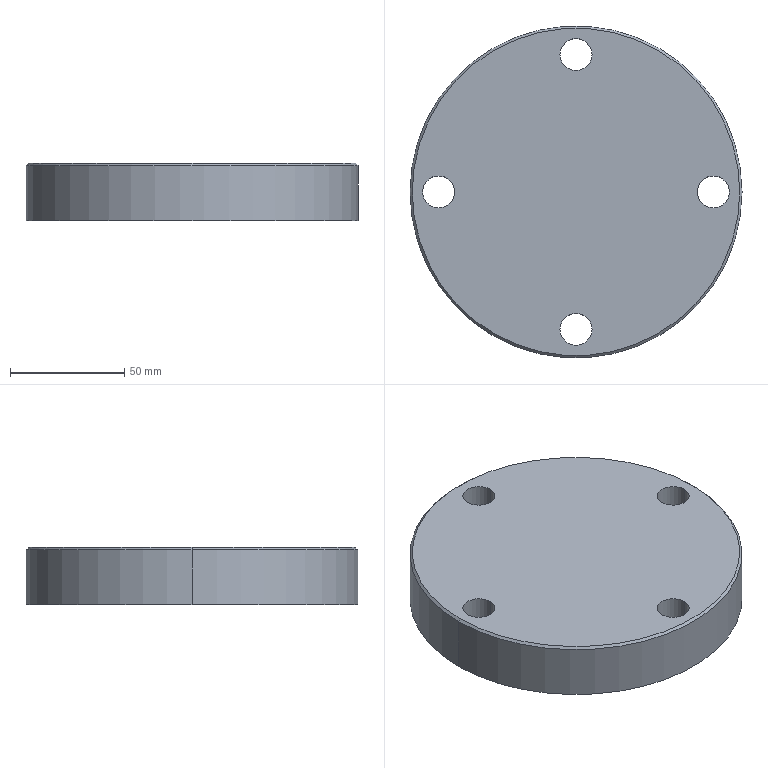Part | SolidWorks | features Chamfer 2, ICE 2, Extrusion 1 | 1 solid | 25 faces | box 145 x 145 x 25 mm | volume 302931 mm3 | cylinder 13 | plane 7 | cone 5 | commonest cylinder face diameters 14 x8 97 x3 145 x2
STEP:
#1=CARTESIAN_POINT('',(-48.5,0.,1.));
#2=VERTEX_POINT('',#1);
#3=CARTESIAN_POINT('',(-32.5,36.,1.));
#4=VERTEX_POINT('',#3);
#5=CARTESIAN_POINT('',(0.,0.,1.));
#6=DIRECTION('',(0.,0.,-1.));
#7=DIRECTION('',(1.,0.,0.));
#8=AXIS2_PLACEMENT_3D('',#5,#6,#7);
#9=CIRCLE('',#8,48.5);
#10=EDGE_CURVE('',#2,#4,#9,.T.);
#11=ORIENTED_EDGE('',*,*,#10,.F.);
#12=CARTESIAN_POINT('',(-49.5,0.,0.));
#13=VERTEX_POINT('',#12);
#14=CARTESIAN_POINT('',(-48.5,0.,1.));
#15=DIRECTION('',(-0.7071,0.,-0.7071));
#16=VECTOR('',#15,1000.);
#17=LINE('',#14,#16);
#18=EDGE_CURVE('',#2,#13,#17,.T.);
#19=ORIENTED_EDGE('',*,*,#18,.T.);
#20=CARTESIAN_POINT('',(-32.882,37.,0.));
#21=VERTEX_POINT('',#20);
#22=CARTESIAN_POINT('',(0.,0.,0.));
#23=DIRECTION('',(0.,0.,1.));
#24=DIRECTION('',(1.,0.,0.));
#25=AXIS2_PLACEMENT_3D('',#22,#23,#24);
#26=CIRCLE('',#25,49.5);
#27=EDGE_CURVE('',#21,#13,#26,.T.);
#28=ORIENTED_EDGE('',*,*,#27,.F.);
#29=CARTESIAN_POINT('',(-32.5,36.,1.));
#30=CARTESIAN_POINT('',(-32.628,36.333,0.6668));
#31=CARTESIAN_POINT('',(-32.756,36.667,0.3335));
#32=CARTESIAN_POINT('',(-32.882,37.,0.));
#33=B_SPLINE_CURVE_WITH_KNOTS('',3,(#29,#30,#31,#32),.UNSPECIFIED.,.F.,.F.,(4,4),(0.,0.001465),.UNSPECIFIED.);
#34=EDGE_CURVE('',#4,#21,#33,.T.);
#35=ORIENTED_EDGE('',*,*,#34,.F.);
#36=EDGE_LOOP('',(#11,#19,#28,#35));
#37=FACE_OUTER_BOUND('',#36,.T.);
#38=CARTESIAN_POINT('',(0.,0.,1.));
#39=DIRECTION('',(0.,0.,-1.));
#40=DIRECTION('',(-1.,0.,0.));
#41=AXIS2_PLACEMENT_3D('',#38,#39,#40);
#42=CONICAL_SURFACE('',#41,48.5,0.7854);
#43=ADVANCED_FACE('',(#37),#42,.F.);
#44=CARTESIAN_POINT('',(71.5,0.,25.));
#45=VERTEX_POINT('',#44);
#46=CARTESIAN_POINT('',(-71.5,0.,25.));
#47=VERTEX_POINT('',#46);
#48=CARTESIAN_POINT('',(0.,0.,25.));
#49=DIRECTION('',(0.,0.,1.));
#50=DIRECTION('',(1.,0.,0.));
#51=AXIS2_PLACEMENT_3D('',#48,#49,#50);
#52=CIRCLE('',#51,71.5);
#53=EDGE_CURVE('',#45,#47,#52,.T.);
#54=ORIENTED_EDGE('',*,*,#53,.F.);
#55=CARTESIAN_POINT('',(72.5,0.,24.));
#56=VERTEX_POINT('',#55);
#57=CARTESIAN_POINT('',(71.5,0.,25.));
#58=DIRECTION('',(0.7071,0.,-0.7071));
#59=VECTOR('',#58,1000.);
#60=LINE('',#57,#59);
#61=EDGE_CURVE('',#45,#56,#60,.T.);
#62=ORIENTED_EDGE('',*,*,#61,.T.);
#63=CARTESIAN_POINT('',(-72.5,0.,24.));
#64=VERTEX_POINT('',#63);
#65=CARTESIAN_POINT('',(0.,0.,24.));
#66=DIRECTION('',(0.,0.,-1.));
#67=DIRECTION('',(1.,0.,0.));
#68=AXIS2_PLACEMENT_3D('',#65,#66,#67);
#69=CIRCLE('',#68,72.5);
#70=EDGE_CURVE('',#64,#56,#69,.T.);
#71=ORIENTED_EDGE('',*,*,#70,.F.);
#72=CARTESIAN_POINT('',(-71.5,0.,25.));
#73=DIRECTION('',(-0.7071,0.,-0.7071));
#74=VECTOR('',#73,1000.);
#75=LINE('',#72,#74);
#76=EDGE_CURVE('',#47,#64,#75,.T.);
#77=ORIENTED_EDGE('',*,*,#76,.F.);
#78=EDGE_LOOP('',(#54,#62,#71,#77));
#79=FACE_OUTER_BOUND('',#78,.T.);
#80=CARTESIAN_POINT('',(0.,0.,25.));
#81=DIRECTION('',(0.,0.,-1.));
#82=DIRECTION('',(-1.,0.,0.));
#83=AXIS2_PLACEMENT_3D('',#80,#81,#82);
#84=CONICAL_SURFACE('',#83,71.5,0.7854);
#85=ADVANCED_FACE('',(#79),#84,.T.);
#86=CARTESIAN_POINT('',(-48.5,0.,15.));
#87=VERTEX_POINT('',#86);
#88=CARTESIAN_POINT('',(-32.5,36.,15.));
#89=VERTEX_POINT('',#88);
#90=CARTESIAN_POINT('',(0.,0.,15.));
#91=DIRECTION('',(0.,0.,-1.));
#92=DIRECTION('',(-1.,0.,0.));
#93=AXIS2_PLACEMENT_3D('',#90,#91,#92);
#94=CIRCLE('',#93,48.5);
#95=EDGE_CURVE('',#87,#89,#94,.T.);
#96=ORIENTED_EDGE('',*,*,#95,.F.);
#97=CARTESIAN_POINT('',(-48.5,0.,15.));
#98=DIRECTION('',(0.,0.,-1.));
#99=VECTOR('',#98,1000.);
#100=LINE('',#97,#99);
#101=EDGE_CURVE('',#87,#2,#100,.T.);
#102=ORIENTED_EDGE('',*,*,#101,.T.);
#103=ORIENTED_EDGE('',*,*,#10,.T.);
#104=CARTESIAN_POINT('',(-32.5,36.,15.));
#105=DIRECTION('',(0.,0.,-1.));
#106=VECTOR('',#105,1000.);
#107=LINE('',#104,#106);
#108=EDGE_CURVE('',#89,#4,#107,.T.);
#109=ORIENTED_EDGE('',*,*,#108,.F.);
#110=EDGE_LOOP('',(#96,#102,#103,#109));
#111=FACE_OUTER_BOUND('',#110,.T.);
#112=CARTESIAN_POINT('',(0.,0.,15.));
#113=DIRECTION('',(0.,0.,-1.));
#114=DIRECTION('',(-1.,0.,0.));
#115=AXIS2_PLACEMENT_3D('',#112,#113,#114);
#116=CYLINDRICAL_SURFACE('',#115,48.5);
#117=ADVANCED_FACE('',(#111),#116,.F.);
#118=CARTESIAN_POINT('',(53.,0.,0.));
#119=VERTEX_POINT('',#118);
#120=CARTESIAN_POINT('',(67.,0.,0.));
#121=VERTEX_POINT('',#120);
#122=CARTESIAN_POINT('',(60.,0.,0.));
#123=DIRECTION('',(0.,0.,1.));
#124=DIRECTION('',(1.,0.,0.));
#125=AXIS2_PLACEMENT_3D('',#122,#123,#124);
#126=CIRCLE('',#125,7.);
#127=EDGE_CURVE('',#119,#121,#126,.T.);
#128=ORIENTED_EDGE('',*,*,#127,.F.);
#129=CARTESIAN_POINT('',(53.,0.,25.));
#130=VERTEX_POINT('',#129);
#131=CARTESIAN_POINT('',(53.,0.,0.));
#132=DIRECTION('',(0.,0.,1.));
#133=VECTOR('',#132,1000.);
#134=LINE('',#131,#133);
#135=EDGE_CURVE('',#119,#130,#134,.T.);
#136=ORIENTED_EDGE('',*,*,#135,.T.);
#137=CARTESIAN_POINT('',(67.,0.,25.));
#138=VERTEX_POINT('',#137);
#139=CARTESIAN_POINT('',(60.,0.,25.));
#140=DIRECTION('',(0.,0.,1.));
#141=DIRECTION('',(1.,0.,0.));
#142=AXIS2_PLACEMENT_3D('',#139,#140,#141);
#143=CIRCLE('',#142,7.);
#144=EDGE_CURVE('',#130,#138,#143,.T.);
#145=ORIENTED_EDGE('',*,*,#144,.T.);
#146=CARTESIAN_POINT('',(67.,0.,0.));
#147=DIRECTION('',(0.,0.,1.));
#148=VECTOR('',#147,1000.);
#149=LINE('',#146,#148);
#150=EDGE_CURVE('',#121,#138,#149,.T.);
#151=ORIENTED_EDGE('',*,*,#150,.F.);
#152=EDGE_LOOP('',(#128,#136,#145,#151));
#153=FACE_OUTER_BOUND('',#152,.T.);
#154=CARTESIAN_POINT('',(60.,0.,0.));
#155=DIRECTION('',(0.,0.,1.));
#156=DIRECTION('',(1.,0.,0.));
#157=AXIS2_PLACEMENT_3D('',#154,#155,#156);
#158=CYLINDRICAL_SURFACE('',#157,7.);
#159=ADVANCED_FACE('',(#153),#158,.F.);
#160=CARTESIAN_POINT('',(-7.,-60.,0.));
#161=VERTEX_POINT('',#160);
#162=CARTESIAN_POINT('',(7.,-60.,0.));
#163=VERTEX_POINT('',#162);
#164=CARTESIAN_POINT('',(0.,-60.,0.));
#165=DIRECTION('',(0.,0.,1.));
#166=DIRECTION('',(1.,0.,0.));
#167=AXIS2_PLACEMENT_3D('',#164,#165,#166);
#168=CIRCLE('',#167,7.);
#169=EDGE_CURVE('',#161,#163,#168,.T.);
#170=ORIENTED_EDGE('',*,*,#169,.F.);
#171=CARTESIAN_POINT('',(-7.,-60.,25.));
#172=VERTEX_POINT('',#171);
#173=CARTESIAN_POINT('',(-7.,-60.,0.));
#174=DIRECTION('',(0.,0.,1.));
#175=VECTOR('',#174,1000.);
#176=LINE('',#173,#175);
#177=EDGE_CURVE('',#161,#172,#176,.T.);
#178=ORIENTED_EDGE('',*,*,#177,.T.);
#179=CARTESIAN_POINT('',(7.,-60.,25.));
#180=VERTEX_POINT('',#179);
#181=CARTESIAN_POINT('',(0.,-60.,25.));
#182=DIRECTION('',(0.,0.,1.));
#183=DIRECTION('',(1.,0.,0.));
#184=AXIS2_PLACEMENT_3D('',#181,#182,#183);
#185=CIRCLE('',#184,7.);
#186=EDGE_CURVE('',#172,#180,#185,.T.);
#187=ORIENTED_EDGE('',*,*,#186,.T.);
#188=CARTESIAN_POINT('',(7.,-60.,0.));
#189=DIRECTION('',(0.,0.,1.));
#190=VECTOR('',#189,1000.);
#191=LINE('',#188,#190);
#192=EDGE_CURVE('',#163,#180,#191,.T.);
#193=ORIENTED_EDGE('',*,*,#192,.F.);
#194=EDGE_LOOP('',(#170,#178,#187,#193));
#195=FACE_OUTER_BOUND('',#194,.T.);
#196=CARTESIAN_POINT('',(0.,-60.,0.));
#197=DIRECTION('',(0.,0.,1.));
#198=DIRECTION('',(1.,0.,0.));
#199=AXIS2_PLACEMENT_3D('',#196,#197,#198);
#200=CYLINDRICAL_SURFACE('',#199,7.);
#201=ADVANCED_FACE('',(#195),#200,.F.);
#202=CARTESIAN_POINT('',(-67.,0.,0.));
#203=VERTEX_POINT('',#202);
#204=CARTESIAN_POINT('',(-53.,0.,0.));
#205=VERTEX_POINT('',#204);
#206=CARTESIAN_POINT('',(-60.,0.,0.));
#207=DIRECTION('',(0.,0.,1.));
#208=DIRECTION('',(1.,0.,0.));
#209=AXIS2_PLACEMENT_3D('',#206,#207,#208);
#210=CIRCLE('',#209,7.);
#211=EDGE_CURVE('',#203,#205,#210,.T.);
#212=ORIENTED_EDGE('',*,*,#211,.F.);
#213=CARTESIAN_POINT('',(-67.,0.,25.));
#214=VERTEX_POINT('',#213);
#215=CARTESIAN_POINT('',(-67.,0.,0.));
#216=DIRECTION('',(0.,0.,1.));
#217=VECTOR('',#216,1000.);
#218=LINE('',#215,#217);
#219=EDGE_CURVE('',#203,#214,#218,.T.);
#220=ORIENTED_EDGE('',*,*,#219,.T.);
#221=CARTESIAN_POINT('',(-53.,0.,25.));
#222=VERTEX_POINT('',#221);
#223=CARTESIAN_POINT('',(-60.,0.,25.));
#224=DIRECTION('',(0.,0.,1.));
#225=DIRECTION('',(1.,0.,0.));
#226=AXIS2_PLACEMENT_3D('',#223,#224,#225);
#227=CIRCLE('',#226,7.);
#228=EDGE_CURVE('',#214,#222,#227,.T.);
#229=ORIENTED_EDGE('',*,*,#228,.T.);
#230=CARTESIAN_POINT('',(-53.,0.,0.));
#231=DIRECTION('',(0.,0.,1.));
#232=VECTOR('',#231,1000.);
#233=LINE('',#230,#232);
#234=EDGE_CURVE('',#205,#222,#233,.T.);
#235=ORIENTED_EDGE('',*,*,#234,.F.);
#236=EDGE_LOOP('',(#212,#220,#229,#235));
#237=FACE_OUTER_BOUND('',#236,.T.);
#238=CARTESIAN_POINT('',(-60.,0.,0.));
#239=DIRECTION('',(0.,0.,1.));
#240=DIRECTION('',(1.,0.,0.));
#241=AXIS2_PLACEMENT_3D('',#238,#239,#240);
#242=CYLINDRICAL_SURFACE('',#241,7.);
#243=ADVANCED_FACE('',(#237),#242,.F.);
#244=CARTESIAN_POINT('',(-7.,60.,0.));
#245=VERTEX_POINT('',#244);
#246=CARTESIAN_POINT('',(7.,60.,0.));
#247=VERTEX_POINT('',#246);
#248=CARTESIAN_POINT('',(0.,60.,0.));
#249=DIRECTION('',(0.,0.,1.));
#250=DIRECTION('',(1.,0.,0.));
#251=AXIS2_PLACEMENT_3D('',#248,#249,#250);
#252=CIRCLE('',#251,7.);
#253=EDGE_CURVE('',#245,#247,#252,.T.);
#254=ORIENTED_EDGE('',*,*,#253,.F.);
#255=CARTESIAN_POINT('',(-7.,60.,25.));
#256=VERTEX_POINT('',#255);
#257=CARTESIAN_POINT('',(-7.,60.,0.));
#258=DIRECTION('',(0.,0.,1.));
#259=VECTOR('',#258,1000.);
#260=LINE('',#257,#259);
#261=EDGE_CURVE('',#245,#256,#260,.T.);
#262=ORIENTED_EDGE('',*,*,#261,.T.);
#263=CARTESIAN_POINT('',(7.,60.,25.));
#264=VERTEX_POINT('',#263);
#265=CARTESIAN_POINT('',(0.,60.,25.));
#266=DIRECTION('',(0.,0.,1.));
#267=DIRECTION('',(1.,0.,0.));
#268=AXIS2_PLACEMENT_3D('',#265,#266,#267);
#269=CIRCLE('',#268,7.);
#270=EDGE_CURVE('',#256,#264,#269,.T.);
#271=ORIENTED_EDGE('',*,*,#270,.T.);
#272=CARTESIAN_POINT('',(7.,60.,0.));
#273=DIRECTION('',(0.,0.,1.));
#274=VECTOR('',#273,1000.);
#275=LINE('',#272,#274);
#276=EDGE_CURVE('',#247,#264,#275,.T.);
#277=ORIENTED_EDGE('',*,*,#276,.F.);
#278=EDGE_LOOP('',(#254,#262,#271,#277));
#279=FACE_OUTER_BOUND('',#278,.T.);
#280=CARTESIAN_POINT('',(0.,60.,0.));
#281=DIRECTION('',(0.,0.,1.));
#282=DIRECTION('',(1.,0.,0.));
#283=AXIS2_PLACEMENT_3D('',#280,#281,#282);
#284=CYLINDRICAL_SURFACE('',#283,7.);
#285=ADVANCED_FACE('',(#279),#284,.F.);
#286=ORIENTED_EDGE('',*,*,#70,.T.);
#287=CARTESIAN_POINT('',(72.5,0.,0.));
#288=VERTEX_POINT('',#287);
#289=CARTESIAN_POINT('',(72.5,0.,25.));
#290=DIRECTION('',(0.,0.,-1.));
#291=VECTOR('',#290,1000.);
#292=LINE('',#289,#291);
#293=EDGE_CURVE('',#56,#288,#292,.T.);
#294=ORIENTED_EDGE('',*,*,#293,.T.);
#295=CARTESIAN_POINT('',(-72.5,0.,0.));
#296=VERTEX_POINT('',#295);
#297=CARTESIAN_POINT('',(0.,0.,0.));
#298=DIRECTION('',(0.,0.,1.));
#299=DIRECTION('',(1.,0.,0.));
#300=AXIS2_PLACEMENT_3D('',#297,#298,#299);
#301=CIRCLE('',#300,72.5);
#302=EDGE_CURVE('',#288,#296,#301,.T.);
#303=ORIENTED_EDGE('',*,*,#302,.T.);
#304=CARTESIAN_POINT('',(-72.5,0.,25.));
#305=DIRECTION('',(0.,0.,-1.));
#306=VECTOR('',#305,1000.);
#307=LINE('',#304,#306);
#308=EDGE_CURVE('',#64,#296,#307,.T.);
#309=ORIENTED_EDGE('',*,*,#308,.F.);
#310=EDGE_LOOP('',(#286,#294,#303,#309));
#311=FACE_OUTER_BOUND('',#310,.T.);
#312=CARTESIAN_POINT('',(0.,0.,25.));
#313=DIRECTION('',(0.,0.,-1.));
#314=DIRECTION('',(-1.,0.,0.));
#315=AXIS2_PLACEMENT_3D('',#312,#313,#314);
#316=CYLINDRICAL_SURFACE('',#315,72.5);
#317=ADVANCED_FACE('',(#311),#316,.T.);
#318=ORIENTED_EDGE('',*,*,#293,.F.);
#319=CARTESIAN_POINT('',(0.,0.,24.));
#320=DIRECTION('',(0.,0.,-1.));
#321=DIRECTION('',(1.,0.,0.));
#322=AXIS2_PLACEMENT_3D('',#319,#320,#321);
#323=CIRCLE('',#322,72.5);
#324=EDGE_CURVE('',#56,#64,#323,.T.);
#325=ORIENTED_EDGE('',*,*,#324,.T.);
#326=ORIENTED_EDGE('',*,*,#308,.T.);
#327=CARTESIAN_POINT('',(0.,0.,0.));
#328=DIRECTION('',(0.,0.,1.));
#329=DIRECTION('',(1.,0.,0.));
#330=AXIS2_PLACEMENT_3D('',#327,#328,#329);
#331=CIRCLE('',#330,72.5);
#332=EDGE_CURVE('',#296,#288,#331,.T.);
#333=ORIENTED_EDGE('',*,*,#332,.T.);
#334=EDGE_LOOP('',(#318,#325,#326,#333));
#335=FACE_OUTER_BOUND('',#334,.T.);
#336=CARTESIAN_POINT('',(0.,0.,25.));
#337=DIRECTION('',(0.,0.,-1.));
#338=DIRECTION('',(-1.,0.,0.));
#339=AXIS2_PLACEMENT_3D('',#336,#337,#338);
#340=CYLINDRICAL_SURFACE('',#339,72.5);
#341=ADVANCED_FACE('',(#335),#340,.T.);
#342=CARTESIAN_POINT('',(0.,0.,25.));
#343=DIRECTION('',(0.,0.,1.));
#344=DIRECTION('',(1.,0.,0.));
#345=AXIS2_PLACEMENT_3D('',#342,#343,#344);
#346=CIRCLE('',#345,71.5);
#347=EDGE_CURVE('',#47,#45,#346,.T.);
#348=ORIENTED_EDGE('',*,*,#347,.T.);
#349=ORIENTED_EDGE('',*,*,#53,.T.);
#350=EDGE_LOOP('',(#348,#349));
#351=FACE_OUTER_BOUND('',#350,.T.);
#352=CARTESIAN_POINT('',(60.,0.,25.));
#353=DIRECTION('',(0.,0.,1.));
#354=DIRECTION('',(1.,0.,0.));
#355=AXIS2_PLACEMENT_3D('',#352,#353,#354);
#356=CIRCLE('',#355,7.);
#357=EDGE_CURVE('',#138,#130,#356,.T.);
#358=ORIENTED_EDGE('',*,*,#357,.F.);
#359=ORIENTED_EDGE('',*,*,#144,.F.);
#360=EDGE_LOOP('',(#358,#359));
#361=FACE_BOUND('',#360,.T.);
#362=CARTESIAN_POINT('',(0.,-60.,25.));
#363=DIRECTION('',(0.,0.,1.));
#364=DIRECTION('',(1.,0.,0.));
#365=AXIS2_PLACEMENT_3D('',#362,#363,#364);
#366=CIRCLE('',#365,7.);
#367=EDGE_CURVE('',#180,#172,#366,.T.);
#368=ORIENTED_EDGE('',*,*,#367,.F.);
#369=ORIENTED_EDGE('',*,*,#186,.F.);
#370=EDGE_LOOP('',(#368,#369));
#371=FACE_BOUND('',#370,.T.);
#372=CARTESIAN_POINT('',(-60.,0.,25.));
#373=DIRECTION('',(0.,0.,1.));
#374=DIRECTION('',(1.,0.,0.));
#375=AXIS2_PLACEMENT_3D('',#372,#373,#374);
#376=CIRCLE('',#375,7.);
#377=EDGE_CURVE('',#222,#214,#376,.T.);
#378=ORIENTED_EDGE('',*,*,#377,.F.);
#379=ORIENTED_EDGE('',*,*,#228,.F.);
#380=EDGE_LOOP('',(#378,#379));
#381=FACE_BOUND('',#380,.T.);
#382=CARTESIAN_POINT('',(0.,60.,25.));
#383=DIRECTION('',(0.,0.,1.));
#384=DIRECTION('',(1.,0.,0.));
#385=AXIS2_PLACEMENT_3D('',#382,#383,#384);
#386=CIRCLE('',#385,7.);
#387=EDGE_CURVE('',#264,#256,#386,.T.);
#388=ORIENTED_EDGE('',*,*,#387,.F.);
#389=ORIENTED_EDGE('',*,*,#270,.F.);
#390=EDGE_LOOP('',(#388,#389));
#391=FACE_BOUND('',#390,.T.);
#392=CARTESIAN_POINT('',(0.,0.,25.));
#393=DIRECTION('',(0.,0.,1.));
#394=DIRECTION('',(1.,0.,0.));
#395=AXIS2_PLACEMENT_3D('',#392,#393,#394);
#396=PLANE('',#395);
#397=ADVANCED_FACE('',(#351,#361,#371,#381,#391),#396,.T.);
#398=CARTESIAN_POINT('',(32.882,-37.,0.));
#399=VERTEX_POINT('',#398);
#400=CARTESIAN_POINT('',(32.882,37.,0.));
#401=VERTEX_POINT('',#400);
#402=CARTESIAN_POINT('',(0.,0.,0.));
#403=DIRECTION('',(0.,0.,1.));
#404=DIRECTION('',(1.,0.,0.));
#405=AXIS2_PLACEMENT_3D('',#402,#403,#404);
#406=CIRCLE('',#405,49.5);
#407=EDGE_CURVE('',#399,#401,#406,.T.);
#408=ORIENTED_EDGE('',*,*,#407,.T.);
#409=CARTESIAN_POINT('',(0.,37.,0.));
#410=DIRECTION('',(-1.,0.,0.));
#411=VECTOR('',#410,1000.);
#412=LINE('',#409,#411);
#413=EDGE_CURVE('',#401,#21,#412,.T.);
#414=ORIENTED_EDGE('',*,*,#413,.T.);
#415=ORIENTED_EDGE('',*,*,#27,.T.);
#416=CARTESIAN_POINT('',(-32.882,-37.,0.));
#417=VERTEX_POINT('',#416);
#418=CARTESIAN_POINT('',(0.,0.,0.));
#419=DIRECTION('',(0.,0.,1.));
#420=DIRECTION('',(1.,0.,0.));
#421=AXIS2_PLACEMENT_3D('',#418,#419,#420);
#422=CIRCLE('',#421,49.5);
#423=EDGE_CURVE('',#13,#417,#422,.T.);
#424=ORIENTED_EDGE('',*,*,#423,.T.);
#425=CARTESIAN_POINT('',(0.,-37.,0.));
#426=DIRECTION('',(1.,0.,0.));
#427=VECTOR('',#426,1000.);
#428=LINE('',#425,#427);
#429=EDGE_CURVE('',#417,#399,#428,.T.);
#430=ORIENTED_EDGE('',*,*,#429,.T.);
#431=EDGE_LOOP('',(#408,#414,#415,#424,#430));
#432=FACE_BOUND('',#431,.T.);
#433=CARTESIAN_POINT('',(60.,0.,0.));
#434=DIRECTION('',(0.,0.,1.));
#435=DIRECTION('',(1.,0.,0.));
#436=AXIS2_PLACEMENT_3D('',#433,#434,#435);
#437=CIRCLE('',#436,7.);
#438=EDGE_CURVE('',#121,#119,#437,.T.);
#439=ORIENTED_EDGE('',*,*,#438,.T.);
#440=ORIENTED_EDGE('',*,*,#127,.T.);
#441=EDGE_LOOP('',(#439,#440));
#442=FACE_BOUND('',#441,.T.);
#443=CARTESIAN_POINT('',(0.,-60.,0.));
#444=DIRECTION('',(0.,0.,1.));
#445=DIRECTION('',(1.,0.,0.));
#446=AXIS2_PLACEMENT_3D('',#443,#444,#445);
#447=CIRCLE('',#446,7.);
#448=EDGE_CURVE('',#163,#161,#447,.T.);
#449=ORIENTED_EDGE('',*,*,#448,.T.);
#450=ORIENTED_EDGE('',*,*,#169,.T.);
#451=EDGE_LOOP('',(#449,#450));
#452=FACE_BOUND('',#451,.T.);
#453=CARTESIAN_POINT('',(-60.,0.,0.));
#454=DIRECTION('',(0.,0.,1.));
#455=DIRECTION('',(1.,0.,0.));
#456=AXIS2_PLACEMENT_3D('',#453,#454,#455);
#457=CIRCLE('',#456,7.);
#458=EDGE_CURVE('',#205,#203,#457,.T.);
#459=ORIENTED_EDGE('',*,*,#458,.T.);
#460=ORIENTED_EDGE('',*,*,#211,.T.);
#461=EDGE_LOOP('',(#459,#460));
#462=FACE_BOUND('',#461,.T.);
#463=CARTESIAN_POINT('',(0.,60.,0.));
#464=DIRECTION('',(0.,0.,1.));
#465=DIRECTION('',(1.,0.,0.));
#466=AXIS2_PLACEMENT_3D('',#463,#464,#465);
#467=CIRCLE('',#466,7.);
#468=EDGE_CURVE('',#247,#245,#467,.T.);
#469=ORIENTED_EDGE('',*,*,#468,.T.);
#470=ORIENTED_EDGE('',*,*,#253,.T.);
#471=EDGE_LOOP('',(#469,#470));
#472=FACE_BOUND('',#471,.T.);
#473=ORIENTED_EDGE('',*,*,#332,.F.);
#474=ORIENTED_EDGE('',*,*,#302,.F.);
#475=EDGE_LOOP('',(#473,#474));
#476=FACE_OUTER_BOUND('',#475,.T.);
#477=CARTESIAN_POINT('',(0.,0.,0.));
#478=DIRECTION('',(0.,0.,1.));
#479=DIRECTION('',(1.,0.,0.));
#480=AXIS2_PLACEMENT_3D('',#477,#478,#479);
#481=PLANE('',#480);
#482=ADVANCED_FACE('',(#432,#442,#452,#462,#472,#476),#481,.F.);
#483=ORIENTED_EDGE('',*,*,#261,.F.);
#484=ORIENTED_EDGE('',*,*,#468,.F.);
#485=ORIENTED_EDGE('',*,*,#276,.T.);
#486=ORIENTED_EDGE('',*,*,#387,.T.);
#487=EDGE_LOOP('',(#483,#484,#485,#486));
#488=FACE_OUTER_BOUND('',#487,.T.);
#489=CARTESIAN_POINT('',(0.,60.,0.));
#490=DIRECTION('',(0.,0.,1.));
#491=DIRECTION('',(1.,0.,0.));
#492=AXIS2_PLACEMENT_3D('',#489,#490,#491);
#493=CYLINDRICAL_SURFACE('',#492,7.);
#494=ADVANCED_FACE('',(#488),#493,.F.);
#495=ORIENTED_EDGE('',*,*,#219,.F.);
#496=ORIENTED_EDGE('',*,*,#458,.F.);
#497=ORIENTED_EDGE('',*,*,#234,.T.);
#498=ORIENTED_EDGE('',*,*,#377,.T.);
#499=EDGE_LOOP('',(#495,#496,#497,#498));
#500=FACE_OUTER_BOUND('',#499,.T.);
#501=CARTESIAN_POINT('',(-60.,0.,0.));
#502=DIRECTION('',(0.,0.,1.));
#503=DIRECTION('',(1.,0.,0.));
#504=AXIS2_PLACEMENT_3D('',#501,#502,#503);
#505=CYLINDRICAL_SURFACE('',#504,7.);
#506=ADVANCED_FACE('',(#500),#505,.F.);
#507=ORIENTED_EDGE('',*,*,#177,.F.);
#508=ORIENTED_EDGE('',*,*,#448,.F.);
#509=ORIENTED_EDGE('',*,*,#192,.T.);
#510=ORIENTED_EDGE('',*,*,#367,.T.);
#511=EDGE_LOOP('',(#507,#508,#509,#510));
#512=FACE_OUTER_BOUND('',#511,.T.);
#513=CARTESIAN_POINT('',(0.,-60.,0.));
#514=DIRECTION('',(0.,0.,1.));
#515=DIRECTION('',(1.,0.,0.));
#516=AXIS2_PLACEMENT_3D('',#513,#514,#515);
#517=CYLINDRICAL_SURFACE('',#516,7.);
#518=ADVANCED_FACE('',(#512),#517,.F.);
#519=ORIENTED_EDGE('',*,*,#135,.F.);
#520=ORIENTED_EDGE('',*,*,#438,.F.);
#521=ORIENTED_EDGE('',*,*,#150,.T.);
#522=ORIENTED_EDGE('',*,*,#357,.T.);
#523=EDGE_LOOP('',(#519,#520,#521,#522));
#524=FACE_OUTER_BOUND('',#523,.T.);
#525=CARTESIAN_POINT('',(60.,0.,0.));
#526=DIRECTION('',(0.,0.,1.));
#527=DIRECTION('',(1.,0.,0.));
#528=AXIS2_PLACEMENT_3D('',#525,#526,#527);
#529=CYLINDRICAL_SURFACE('',#528,7.);
#530=ADVANCED_FACE('',(#524),#529,.F.);
#531=CARTESIAN_POINT('',(32.5,36.,15.));
#532=VERTEX_POINT('',#531);
#533=CARTESIAN_POINT('',(32.5,36.,1.));
#534=VERTEX_POINT('',#533);
#535=CARTESIAN_POINT('',(32.5,36.,15.));
#536=DIRECTION('',(0.,0.,-1.));
#537=VECTOR('',#536,1000.);
#538=LINE('',#535,#537);
#539=EDGE_CURVE('',#532,#534,#538,.T.);
#540=ORIENTED_EDGE('',*,*,#539,.T.);
#541=CARTESIAN_POINT('',(32.5,-36.,1.));
#542=VERTEX_POINT('',#541);
#543=CARTESIAN_POINT('',(0.,0.,1.));
#544=DIRECTION('',(0.,0.,-1.));
#545=DIRECTION('',(1.,0.,0.));
#546=AXIS2_PLACEMENT_3D('',#543,#544,#545);
#547=CIRCLE('',#546,48.5);
#548=EDGE_CURVE('',#534,#542,#547,.T.);
#549=ORIENTED_EDGE('',*,*,#548,.T.);
#550=CARTESIAN_POINT('',(32.5,-36.,15.));
#551=VERTEX_POINT('',#550);
#552=CARTESIAN_POINT('',(32.5,-36.,15.));
#553=DIRECTION('',(0.,0.,-1.));
#554=VECTOR('',#553,1000.);
#555=LINE('',#552,#554);
#556=EDGE_CURVE('',#551,#542,#555,.T.);
#557=ORIENTED_EDGE('',*,*,#556,.F.);
#558=CARTESIAN_POINT('',(0.,0.,15.));
#559=DIRECTION('',(0.,0.,-1.));
#560=DIRECTION('',(-1.,0.,0.));
#561=AXIS2_PLACEMENT_3D('',#558,#559,#560);
#562=CIRCLE('',#561,48.5);
#563=EDGE_CURVE('',#532,#551,#562,.T.);
#564=ORIENTED_EDGE('',*,*,#563,.F.);
#565=EDGE_LOOP('',(#540,#549,#557,#564));
#566=FACE_OUTER_BOUND('',#565,.T.);
#567=CARTESIAN_POINT('',(0.,0.,15.));
#568=DIRECTION('',(0.,0.,-1.));
#569=DIRECTION('',(-1.,0.,0.));
#570=AXIS2_PLACEMENT_3D('',#567,#568,#569);
#571=CYLINDRICAL_SURFACE('',#570,48.5);
#572=ADVANCED_FACE('',(#566),#571,.F.);
#573=ORIENTED_EDGE('',*,*,#108,.T.);
#574=CARTESIAN_POINT('',(32.5,36.,1.));
#575=DIRECTION('',(1.,0.,0.));
#576=VECTOR('',#575,1000.);
#577=LINE('',#574,#576);
#578=EDGE_CURVE('',#4,#534,#577,.T.);
#579=ORIENTED_EDGE('',*,*,#578,.T.);
#580=ORIENTED_EDGE('',*,*,#539,.F.);
#581=CARTESIAN_POINT('',(32.5,36.,15.));
#582=DIRECTION('',(1.,0.,0.));
#583=VECTOR('',#582,1000.);
#584=LINE('',#581,#583);
#585=EDGE_CURVE('',#89,#532,#584,.T.);
#586=ORIENTED_EDGE('',*,*,#585,.F.);
#587=EDGE_LOOP('',(#573,#579,#580,#586));
#588=FACE_OUTER_BOUND('',#587,.T.);
#589=CARTESIAN_POINT('',(32.5,36.,15.));
#590=DIRECTION('',(0.,1.,0.));
#591=DIRECTION('',(0.,0.,1.));
#592=AXIS2_PLACEMENT_3D('',#589,#590,#591);
#593=PLANE('',#592);
#594=ADVANCED_FACE('',(#588),#593,.F.);
#595=ORIENTED_EDGE('',*,*,#101,.F.);
#596=CARTESIAN_POINT('',(-32.5,-36.,15.));
#597=VERTEX_POINT('',#596);
#598=CARTESIAN_POINT('',(0.,0.,15.));
#599=DIRECTION('',(0.,0.,-1.));
#600=DIRECTION('',(-1.,0.,0.));
#601=AXIS2_PLACEMENT_3D('',#598,#599,#600);
#602=CIRCLE('',#601,48.5);
#603=EDGE_CURVE('',#597,#87,#602,.T.);
#604=ORIENTED_EDGE('',*,*,#603,.F.);
#605=CARTESIAN_POINT('',(-32.5,-36.,1.));
#606=VERTEX_POINT('',#605);
#607=CARTESIAN_POINT('',(-32.5,-36.,15.));
#608=DIRECTION('',(0.,0.,-1.));
#609=VECTOR('',#608,1000.);
#610=LINE('',#607,#609);
#611=EDGE_CURVE('',#597,#606,#610,.T.);
#612=ORIENTED_EDGE('',*,*,#611,.T.);
#613=CARTESIAN_POINT('',(0.,0.,1.));
#614=DIRECTION('',(0.,0.,-1.));
#615=DIRECTION('',(1.,0.,0.));
#616=AXIS2_PLACEMENT_3D('',#613,#614,#615);
#617=CIRCLE('',#616,48.5);
#618=EDGE_CURVE('',#606,#2,#617,.T.);
#619=ORIENTED_EDGE('',*,*,#618,.T.);
#620=EDGE_LOOP('',(#595,#604,#612,#619));
#621=FACE_OUTER_BOUND('',#620,.T.);
#622=CARTESIAN_POINT('',(0.,0.,15.));
#623=DIRECTION('',(0.,0.,-1.));
#624=DIRECTION('',(-1.,0.,0.));
#625=AXIS2_PLACEMENT_3D('',#622,#623,#624);
#626=CYLINDRICAL_SURFACE('',#625,48.5);
#627=ADVANCED_FACE('',(#621),#626,.F.);
#628=ORIENTED_EDGE('',*,*,#556,.T.);
#629=CARTESIAN_POINT('',(32.5,-36.,1.));
#630=DIRECTION('',(-1.,0.,0.));
#631=VECTOR('',#630,1000.);
#632=LINE('',#629,#631);
#633=EDGE_CURVE('',#542,#606,#632,.T.);
#634=ORIENTED_EDGE('',*,*,#633,.T.);
#635=ORIENTED_EDGE('',*,*,#611,.F.);
#636=CARTESIAN_POINT('',(32.5,-36.,15.));
#637=DIRECTION('',(-1.,0.,0.));
#638=VECTOR('',#637,1000.);
#639=LINE('',#636,#638);
#640=EDGE_CURVE('',#551,#597,#639,.T.);
#641=ORIENTED_EDGE('',*,*,#640,.F.);
#642=EDGE_LOOP('',(#628,#634,#635,#641));
#643=FACE_OUTER_BOUND('',#642,.T.);
#644=CARTESIAN_POINT('',(32.5,-36.,15.));
#645=DIRECTION('',(0.,-1.,0.));
#646=DIRECTION('',(0.,0.,-1.));
#647=AXIS2_PLACEMENT_3D('',#644,#645,#646);
#648=PLANE('',#647);
#649=ADVANCED_FACE('',(#643),#648,.F.);
#650=ORIENTED_EDGE('',*,*,#563,.T.);
#651=ORIENTED_EDGE('',*,*,#640,.T.);
#652=ORIENTED_EDGE('',*,*,#603,.T.);
#653=ORIENTED_EDGE('',*,*,#95,.T.);
#654=ORIENTED_EDGE('',*,*,#585,.T.);
#655=EDGE_LOOP('',(#650,#651,#652,#653,#654));
#656=FACE_OUTER_BOUND('',#655,.T.);
#657=CARTESIAN_POINT('',(0.,0.,15.));
#658=DIRECTION('',(0.,0.,-1.));
#659=DIRECTION('',(-1.,0.,0.));
#660=AXIS2_PLACEMENT_3D('',#657,#658,#659);
#661=PLANE('',#660);
#662=ADVANCED_FACE('',(#656),#661,.T.);
#663=ORIENTED_EDGE('',*,*,#61,.F.);
#664=ORIENTED_EDGE('',*,*,#347,.F.);
#665=ORIENTED_EDGE('',*,*,#76,.T.);
#666=ORIENTED_EDGE('',*,*,#324,.F.);
#667=EDGE_LOOP('',(#663,#664,#665,#666));
#668=FACE_OUTER_BOUND('',#667,.T.);
#669=CARTESIAN_POINT('',(0.,0.,25.));
#670=DIRECTION('',(0.,0.,-1.));
#671=DIRECTION('',(-1.,0.,0.));
#672=AXIS2_PLACEMENT_3D('',#669,#670,#671);
#673=CONICAL_SURFACE('',#672,71.5,0.7854);
#674=ADVANCED_FACE('',(#668),#673,.T.);
#675=CARTESIAN_POINT('',(32.882,-37.,0.));
#676=CARTESIAN_POINT('',(32.756,-36.667,0.3335));
#677=CARTESIAN_POINT('',(32.628,-36.333,0.6668));
#678=CARTESIAN_POINT('',(32.5,-36.,1.));
#679=B_SPLINE_CURVE_WITH_KNOTS('',3,(#675,#676,#677,#678),.UNSPECIFIED.,.F.,.F.,(4,4),(0.,0.001465),.UNSPECIFIED.);
#680=EDGE_CURVE('',#399,#542,#679,.T.);
#681=ORIENTED_EDGE('',*,*,#680,.F.);
#682=ORIENTED_EDGE('',*,*,#429,.F.);
#683=CARTESIAN_POINT('',(-32.5,-36.,1.));
#684=CARTESIAN_POINT('',(-32.628,-36.333,0.6668));
#685=CARTESIAN_POINT('',(-32.756,-36.667,0.3335));
#686=CARTESIAN_POINT('',(-32.882,-37.,0.));
#687=B_SPLINE_CURVE_WITH_KNOTS('',3,(#683,#684,#685,#686),.UNSPECIFIED.,.F.,.F.,(4,4),(0.,0.001465),.UNSPECIFIED.);
#688=EDGE_CURVE('',#606,#417,#687,.T.);
#689=ORIENTED_EDGE('',*,*,#688,.F.);
#690=ORIENTED_EDGE('',*,*,#633,.F.);
#691=EDGE_LOOP('',(#681,#682,#689,#690));
#692=FACE_OUTER_BOUND('',#691,.T.);
#693=CARTESIAN_POINT('',(32.5,-36.,1.));
#694=DIRECTION('',(0.,-0.7071,0.7071));
#695=DIRECTION('',(-1.,0.,0.));
#696=AXIS2_PLACEMENT_3D('',#693,#694,#695);
#697=PLANE('',#696);
#698=ADVANCED_FACE('',(#692),#697,.F.);
#699=ORIENTED_EDGE('',*,*,#18,.F.);
#700=ORIENTED_EDGE('',*,*,#618,.F.);
#701=ORIENTED_EDGE('',*,*,#688,.T.);
#702=ORIENTED_EDGE('',*,*,#423,.F.);
#703=EDGE_LOOP('',(#699,#700,#701,#702));
#704=FACE_OUTER_BOUND('',#703,.T.);
#705=CARTESIAN_POINT('',(0.,0.,1.));
#706=DIRECTION('',(0.,0.,-1.));
#707=DIRECTION('',(-1.,0.,0.));
#708=AXIS2_PLACEMENT_3D('',#705,#706,#707);
#709=CONICAL_SURFACE('',#708,48.5,0.7854);
#710=ADVANCED_FACE('',(#704),#709,.F.);
#711=ORIENTED_EDGE('',*,*,#680,.T.);
#712=ORIENTED_EDGE('',*,*,#548,.F.);
#713=CARTESIAN_POINT('',(32.882,37.,0.));
#714=CARTESIAN_POINT('',(32.756,36.667,0.3335));
#715=CARTESIAN_POINT('',(32.628,36.333,0.6668));
#716=CARTESIAN_POINT('',(32.5,36.,1.));
#717=B_SPLINE_CURVE_WITH_KNOTS('',3,(#713,#714,#715,#716),.UNSPECIFIED.,.F.,.F.,(4,4),(0.,0.001465),.UNSPECIFIED.);
#718=EDGE_CURVE('',#401,#534,#717,.T.);
#719=ORIENTED_EDGE('',*,*,#718,.F.);
#720=ORIENTED_EDGE('',*,*,#407,.F.);
#721=EDGE_LOOP('',(#711,#712,#719,#720));
#722=FACE_OUTER_BOUND('',#721,.T.);
#723=CARTESIAN_POINT('',(0.,0.,1.));
#724=DIRECTION('',(0.,0.,-1.));
#725=DIRECTION('',(-1.,0.,0.));
#726=AXIS2_PLACEMENT_3D('',#723,#724,#725);
#727=CONICAL_SURFACE('',#726,48.5,0.7854);
#728=ADVANCED_FACE('',(#722),#727,.F.);
#729=ORIENTED_EDGE('',*,*,#34,.T.);
#730=ORIENTED_EDGE('',*,*,#413,.F.);
#731=ORIENTED_EDGE('',*,*,#718,.T.);
#732=ORIENTED_EDGE('',*,*,#578,.F.);
#733=EDGE_LOOP('',(#729,#730,#731,#732));
#734=FACE_OUTER_BOUND('',#733,.T.);
#735=CARTESIAN_POINT('',(32.5,36.,1.));
#736=DIRECTION('',(0.,0.7071,0.7071));
#737=DIRECTION('',(1.,0.,0.));
#738=AXIS2_PLACEMENT_3D('',#735,#736,#737);
#739=PLANE('',#738);
#740=ADVANCED_FACE('',(#734),#739,.F.);
#741=CLOSED_SHELL('',(#43,#85,#117,#159,#201,#243,#285,#317,#341,#397,#482,#494,#506,#518,#530,#572,#594,#627,#649,#662,#674,#698,#710,#728,#740));
#742=MANIFOLD_SOLID_BREP('',#741);
#743=CARTESIAN_POINT('',(0.,0.,0.));
#744=DIRECTION('',(0.,0.,1.));
#745=DIRECTION('',(1.,0.,0.));
#746=AXIS2_PLACEMENT_3D('',#743,#744,#745);
#747=(LENGTH_UNIT()NAMED_UNIT(*)SI_UNIT(.MILLI.,.METRE.));
#748=UNCERTAINTY_MEASURE_WITH_UNIT(LENGTH_MEASURE(0.00001),#747,'','');
#749=(NAMED_UNIT(*)PLANE_ANGLE_UNIT()SI_UNIT($,.RADIAN.));
#750=(NAMED_UNIT(*)SI_UNIT($,.STERADIAN.)SOLID_ANGLE_UNIT());
#751=(GEOMETRIC_REPRESENTATION_CONTEXT(3)GLOBAL_UNCERTAINTY_ASSIGNED_CONTEXT((#748))GLOBAL_UNIT_ASSIGNED_CONTEXT((#747,#749,#750))REPRESENTATION_CONTEXT('',''));
#752=ADVANCED_BREP_SHAPE_REPRESENTATION('',(#742,#746),#751);